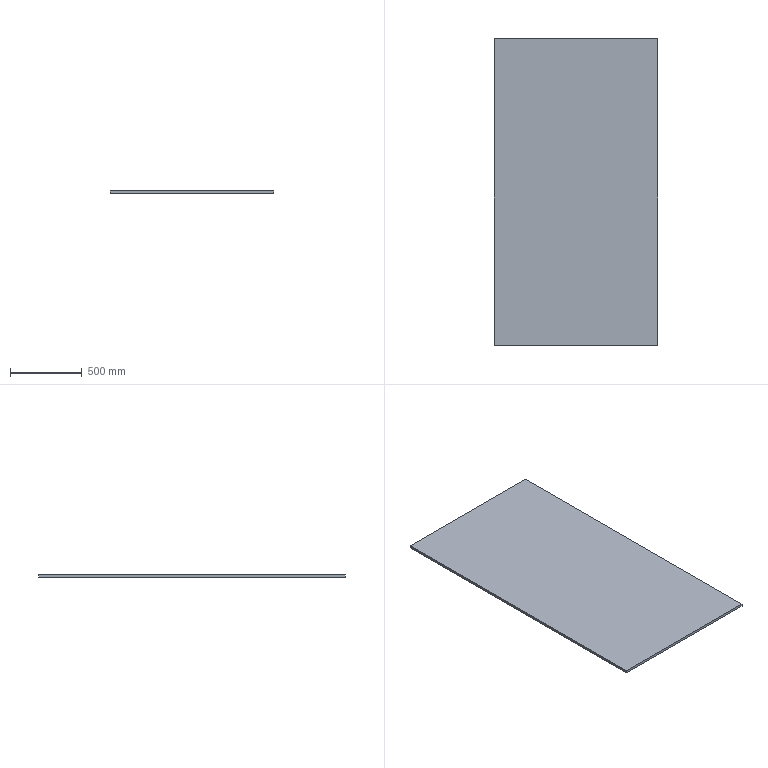Part | SolidWorks | features ICE 2, WeldMemberFeat 1, WeldmentFeature 1 | 1 solid | 6 faces | box 1140 x 2136 x 18 mm | volume 43830720 mm3 | plane 6
STEP:
#1=CARTESIAN_POINT('',(-570.,1068.,9.));
#2=VERTEX_POINT('',#1);
#3=CARTESIAN_POINT('',(-570.,1068.,-9.));
#4=VERTEX_POINT('',#3);
#5=CARTESIAN_POINT('',(-570.,1068.,2430.177));
#6=DIRECTION('',(0.,0.,-1.));
#7=VECTOR('',#6,1000.);
#8=LINE('',#5,#7);
#9=EDGE_CURVE('',#2,#4,#8,.T.);
#10=ORIENTED_EDGE('',*,*,#9,.F.);
#11=CARTESIAN_POINT('',(570.,1068.,9.));
#12=VERTEX_POINT('',#11);
#13=CARTESIAN_POINT('',(-570.,1068.,9.));
#14=DIRECTION('',(1.,0.,0.));
#15=VECTOR('',#14,1000.);
#16=LINE('',#13,#15);
#17=EDGE_CURVE('',#2,#12,#16,.T.);
#18=ORIENTED_EDGE('',*,*,#17,.T.);
#19=CARTESIAN_POINT('',(570.,1068.,-9.));
#20=VERTEX_POINT('',#19);
#21=CARTESIAN_POINT('',(570.,1068.,2430.177));
#22=DIRECTION('',(0.,0.,-1.));
#23=VECTOR('',#22,1000.);
#24=LINE('',#21,#23);
#25=EDGE_CURVE('',#12,#20,#24,.T.);
#26=ORIENTED_EDGE('',*,*,#25,.T.);
#27=CARTESIAN_POINT('',(-570.,1068.,-9.));
#28=DIRECTION('',(1.,0.,0.));
#29=VECTOR('',#28,1000.);
#30=LINE('',#27,#29);
#31=EDGE_CURVE('',#4,#20,#30,.T.);
#32=ORIENTED_EDGE('',*,*,#31,.F.);
#33=EDGE_LOOP('',(#10,#18,#26,#32));
#34=FACE_OUTER_BOUND('',#33,.T.);
#35=CARTESIAN_POINT('',(-570.,1068.,2430.177));
#36=DIRECTION('',(0.,-1.,0.));
#37=DIRECTION('',(0.,0.,-1.));
#38=AXIS2_PLACEMENT_3D('',#35,#36,#37);
#39=PLANE('',#38);
#40=ADVANCED_FACE('',(#34),#39,.F.);
#41=ORIENTED_EDGE('',*,*,#25,.F.);
#42=CARTESIAN_POINT('',(570.,-1068.,9.));
#43=VERTEX_POINT('',#42);
#44=CARTESIAN_POINT('',(570.,1068.,9.));
#45=DIRECTION('',(0.,-1.,0.));
#46=VECTOR('',#45,1000.);
#47=LINE('',#44,#46);
#48=EDGE_CURVE('',#12,#43,#47,.T.);
#49=ORIENTED_EDGE('',*,*,#48,.T.);
#50=CARTESIAN_POINT('',(570.,-1068.,-9.));
#51=VERTEX_POINT('',#50);
#52=CARTESIAN_POINT('',(570.,-1068.,2430.177));
#53=DIRECTION('',(0.,0.,-1.));
#54=VECTOR('',#53,1000.);
#55=LINE('',#52,#54);
#56=EDGE_CURVE('',#43,#51,#55,.T.);
#57=ORIENTED_EDGE('',*,*,#56,.T.);
#58=CARTESIAN_POINT('',(570.,1068.,-9.));
#59=DIRECTION('',(0.,-1.,0.));
#60=VECTOR('',#59,1000.);
#61=LINE('',#58,#60);
#62=EDGE_CURVE('',#20,#51,#61,.T.);
#63=ORIENTED_EDGE('',*,*,#62,.F.);
#64=EDGE_LOOP('',(#41,#49,#57,#63));
#65=FACE_OUTER_BOUND('',#64,.T.);
#66=CARTESIAN_POINT('',(570.,1068.,2430.177));
#67=DIRECTION('',(-1.,0.,0.));
#68=DIRECTION('',(0.,-1.,0.));
#69=AXIS2_PLACEMENT_3D('',#66,#67,#68);
#70=PLANE('',#69);
#71=ADVANCED_FACE('',(#65),#70,.F.);
#72=ORIENTED_EDGE('',*,*,#56,.F.);
#73=CARTESIAN_POINT('',(-570.,-1068.,9.));
#74=VERTEX_POINT('',#73);
#75=CARTESIAN_POINT('',(-570.,-1068.,9.));
#76=DIRECTION('',(-1.,0.,0.));
#77=VECTOR('',#76,1000.);
#78=LINE('',#75,#77);
#79=EDGE_CURVE('',#43,#74,#78,.T.);
#80=ORIENTED_EDGE('',*,*,#79,.T.);
#81=CARTESIAN_POINT('',(-570.,-1068.,-9.));
#82=VERTEX_POINT('',#81);
#83=CARTESIAN_POINT('',(-570.,-1068.,2430.177));
#84=DIRECTION('',(0.,0.,-1.));
#85=VECTOR('',#84,1000.);
#86=LINE('',#83,#85);
#87=EDGE_CURVE('',#74,#82,#86,.T.);
#88=ORIENTED_EDGE('',*,*,#87,.T.);
#89=CARTESIAN_POINT('',(-570.,-1068.,-9.));
#90=DIRECTION('',(-1.,0.,0.));
#91=VECTOR('',#90,1000.);
#92=LINE('',#89,#91);
#93=EDGE_CURVE('',#51,#82,#92,.T.);
#94=ORIENTED_EDGE('',*,*,#93,.F.);
#95=EDGE_LOOP('',(#72,#80,#88,#94));
#96=FACE_OUTER_BOUND('',#95,.T.);
#97=CARTESIAN_POINT('',(-570.,-1068.,2430.177));
#98=DIRECTION('',(0.,1.,0.));
#99=DIRECTION('',(0.,0.,1.));
#100=AXIS2_PLACEMENT_3D('',#97,#98,#99);
#101=PLANE('',#100);
#102=ADVANCED_FACE('',(#96),#101,.F.);
#103=ORIENTED_EDGE('',*,*,#87,.F.);
#104=CARTESIAN_POINT('',(-570.,1068.,9.));
#105=DIRECTION('',(0.,1.,0.));
#106=VECTOR('',#105,1000.);
#107=LINE('',#104,#106);
#108=EDGE_CURVE('',#74,#2,#107,.T.);
#109=ORIENTED_EDGE('',*,*,#108,.T.);
#110=ORIENTED_EDGE('',*,*,#9,.T.);
#111=CARTESIAN_POINT('',(-570.,1068.,-9.));
#112=DIRECTION('',(0.,1.,0.));
#113=VECTOR('',#112,1000.);
#114=LINE('',#111,#113);
#115=EDGE_CURVE('',#82,#4,#114,.T.);
#116=ORIENTED_EDGE('',*,*,#115,.F.);
#117=EDGE_LOOP('',(#103,#109,#110,#116));
#118=FACE_OUTER_BOUND('',#117,.T.);
#119=CARTESIAN_POINT('',(-570.,1068.,2430.177));
#120=DIRECTION('',(1.,0.,0.));
#121=DIRECTION('',(0.,1.,0.));
#122=AXIS2_PLACEMENT_3D('',#119,#120,#121);
#123=PLANE('',#122);
#124=ADVANCED_FACE('',(#118),#123,.F.);
#125=ORIENTED_EDGE('',*,*,#79,.F.);
#126=ORIENTED_EDGE('',*,*,#48,.F.);
#127=ORIENTED_EDGE('',*,*,#17,.F.);
#128=ORIENTED_EDGE('',*,*,#108,.F.);
#129=EDGE_LOOP('',(#125,#126,#127,#128));
#130=FACE_OUTER_BOUND('',#129,.T.);
#131=CARTESIAN_POINT('',(570.,1068.,9.));
#132=DIRECTION('',(0.,0.,-1.));
#133=DIRECTION('',(0.,1.,0.));
#134=AXIS2_PLACEMENT_3D('',#131,#132,#133);
#135=PLANE('',#134);
#136=ADVANCED_FACE('',(#130),#135,.F.);
#137=ORIENTED_EDGE('',*,*,#115,.T.);
#138=ORIENTED_EDGE('',*,*,#31,.T.);
#139=ORIENTED_EDGE('',*,*,#62,.T.);
#140=ORIENTED_EDGE('',*,*,#93,.T.);
#141=EDGE_LOOP('',(#137,#138,#139,#140));
#142=FACE_OUTER_BOUND('',#141,.T.);
#143=CARTESIAN_POINT('',(570.,1038.,-9.));
#144=DIRECTION('',(0.,0.,1.));
#145=DIRECTION('',(0.,-1.,0.));
#146=AXIS2_PLACEMENT_3D('',#143,#144,#145);
#147=PLANE('',#146);
#148=ADVANCED_FACE('',(#142),#147,.F.);
#149=CLOSED_SHELL('',(#40,#71,#102,#124,#136,#148));
#150=MANIFOLD_SOLID_BREP('',#149);
#151=CARTESIAN_POINT('',(0.,0.,0.));
#152=DIRECTION('',(0.,0.,1.));
#153=DIRECTION('',(1.,0.,0.));
#154=AXIS2_PLACEMENT_3D('',#151,#152,#153);
#155=(LENGTH_UNIT()NAMED_UNIT(*)SI_UNIT(.MILLI.,.METRE.));
#156=UNCERTAINTY_MEASURE_WITH_UNIT(LENGTH_MEASURE(0.00001),#155,'','');
#157=(NAMED_UNIT(*)PLANE_ANGLE_UNIT()SI_UNIT($,.RADIAN.));
#158=(NAMED_UNIT(*)SI_UNIT($,.STERADIAN.)SOLID_ANGLE_UNIT());
#159=(GEOMETRIC_REPRESENTATION_CONTEXT(3)GLOBAL_UNCERTAINTY_ASSIGNED_CONTEXT((#156))GLOBAL_UNIT_ASSIGNED_CONTEXT((#155,#157,#158))REPRESENTATION_CONTEXT('',''));
#160=ADVANCED_BREP_SHAPE_REPRESENTATION('',(#150,#154),#159);